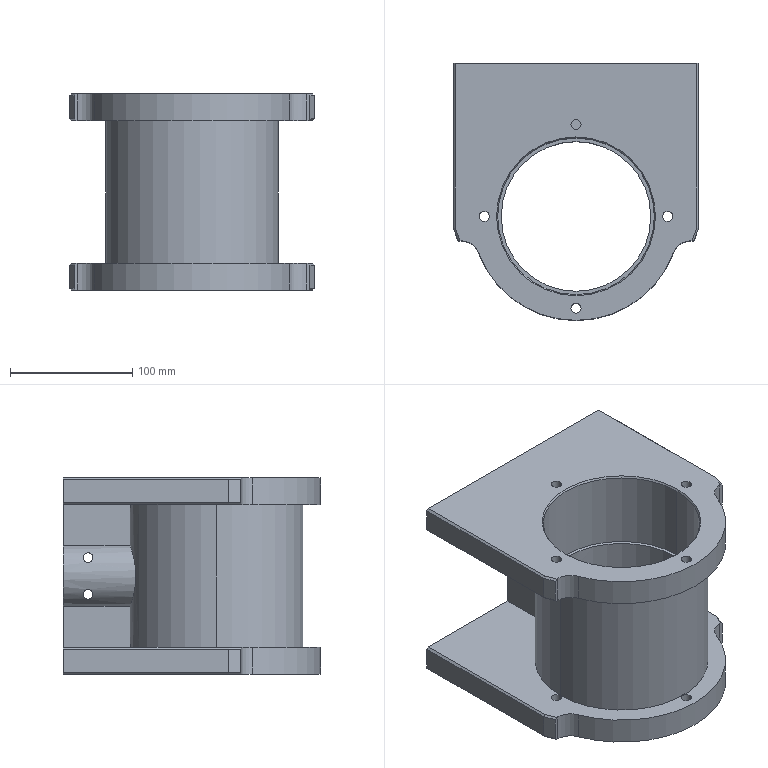Part | SolidWorks | features BaseBody 1 | 1 solid | 89 faces | box 200 x 210 x 160.5 mm | volume 1529038 mm3 | plane 42 | cylinder 41 | cone 6 | commonest cylinder face diameters 8.376 x16 30 x6 8 x4 128 x4 141.3 x3 20 x2